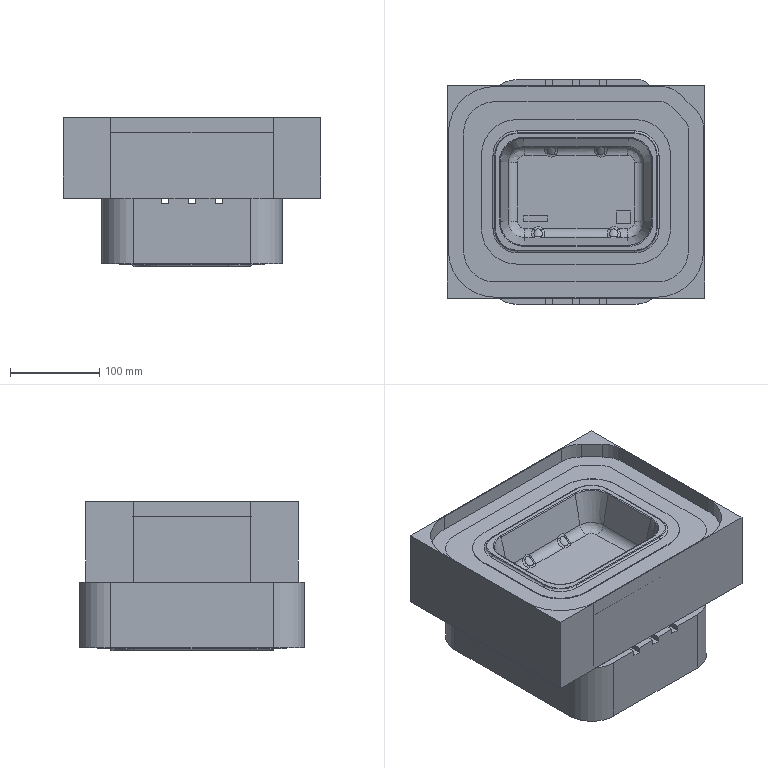NC program | NX | posted with a generic post | part box 287.436 x 251.436 x 167.016 mm
Lines 12510 to 12630 of 118587:
(05 , TOOL : D12)
N25012 M6
N25014 G53
N25016 G17 G0 G90 X48.827 Y111.793 S7000 M3 M8
N25018 G43 Z240.5 H0
N25020 Z75.182
N25022 G94 G1 X86.99 Z73.182 F4000.
N25024 X94.505
N25026 G2 X112.89 Y104.178 R26.
N25028 G1 X129.103 Y87.965
N25030 G2 X136.718 Y69.58 R26.
N25032 G1 Y-65.793
N25034 G2 X90.718 Y-111.793 R46.
N25036 G1 X-90.718
N25038 G2 X-136.718 Y-65.793 R46.
N25040 G1 Y65.793
N25042 G2 X-90.718 Y111.793 R46.
N25044 G1 X86.99
N25046 Y103.393
N25048 X94.505
N25050 G2 X106.95 Y98.238 R17.6
N25052 G1 X123.163 Y82.025
N25054 G2 X128.318 Y69.58 R17.6
N25056 G1 Y-65.793
N25058 G2 X90.718 Y-103.393 R37.6
N25060 G1 X-90.718
N25062 G2 X-128.318 Y-65.793 R37.6
N25064 G1 Y65.793
N25066 G2 X-90.718 Y103.393 R37.6
N25068 G1 X86.99
N25070 Y94.993
N25072 X94.505
N25074 G2 X101.01 Y92.298 R9.2
N25076 G1 X117.223 Y76.085
N25078 G2 X119.918 Y69.58 R9.2
N25080 G1 Y-65.793
N25082 G2 X90.718 Y-94.993 R29.2
N25084 G1 X79.474
N25086 Y-86.593
N25088 G3 X111.518 Y-54.549 R47.097
N25090 G1 Y-65.793
N25092 G2 X90.718 Y-86.593 R20.8
N25094 G1 X79.474
N25096 X73.619 Y-87.901
N25098 G2 X66.301 Y-88.473 R47.097
N25100 G1 X-66.301
N25102 G2 X-73.619 Y-87.901 R47.098
N25104 X-73.975 Y-88.993 R6.
N25106 G1 X73.975
N25108 G2 X73.619 Y-87.901 R6.
N25110 G1 X79.474 Y-86.593
N25112 Y-94.993
N25114 X-90.718
N25116 G2 X-119.918 Y-65.793 R29.2
N25118 G1 Y-54.549
N25120 X-111.518
N25122 G3 X-79.474 Y-86.593 R47.097
N25124 G1 X-90.718
N25126 G2 X-111.518 Y-65.793 R20.8
N25128 G1 Y-54.549
N25130 X-112.826 Y-48.694
N25132 G2 X-113.398 Y-41.376 R47.098
N25134 G1 Y41.376
N25136 G2 X-112.826 Y48.694 R47.097
N25138 X-113.918 Y49.05 R6.
N25140 G1 Y-49.05
N25142 G2 X-112.826 Y-48.694 R6.
N25144 G1 X-111.518 Y-54.549
N25146 X-119.918
N25148 Y65.793
N25150 G2 X-90.718 Y94.993 R29.2
N25152 G1 X-79.474
N25154 Y86.593
N25156 G3 X-111.518 Y54.549 R47.097
N25158 G1 Y65.793
N25160 G2 X-90.718 Y86.593 R20.8
N25162 G1 X-79.474
N25164 Y94.993
N25166 X86.99
N25168 Y86.593
N25170 X94.505
N25172 G2 X95.07 Y86.359 R0.8
N25174 G1 X111.284 Y70.145
N25176 G2 X111.518 Y69.58 R0.8
N25178 G1 Y54.549
N25180 X112.826 Y48.694
N25182 G2 X113.398 Y41.376 R47.097
N25184 G1 Y-41.376
N25186 G2 X112.826 Y-48.694 R47.097
N25188 X113.918 Y-49.05 R6.
N25190 G1 Y49.05
N25192 G2 X112.826 Y48.694 R6.
N25194 G1 X111.518 Y54.549
N25196 G3 X79.474 Y86.593 R47.097
N25198 G1 X73.975 Y88.993
N25200 X-73.975
N25202 G2 X-73.619 Y87.901 R6.
N25204 X-66.301 Y88.473 R47.097
N25206 G1 X66.301
N25208 G2 X73.619 Y87.901 R47.097
N25210 X73.975 Y88.993 R6.
N25212 G1 X79.474 Y86.593
N25214 X79.004 Y84.98
N25216 G2 X111.718 Y41.376 R45.417
N25218 G1 Y-41.376
N25220 G2 X66.301 Y-86.793 R45.418
N25222 G1 X-66.301
N25224 G2 X-111.718 Y-41.376 R45.418
N25226 G1 Y41.376
N25228 G2 X-66.301 Y86.793 R45.417
N25230 G1 X66.301
N25232 G2 X79.004 Y84.98 R45.417
N25234 G1 X79.474 Y86.593
N25236 X86.99
N25238 G3 X89.39 Y88.993 R2.4
N25240 G1 Z74.182
N25242 G0 Z240.5
N25244 M9
N25246 M5